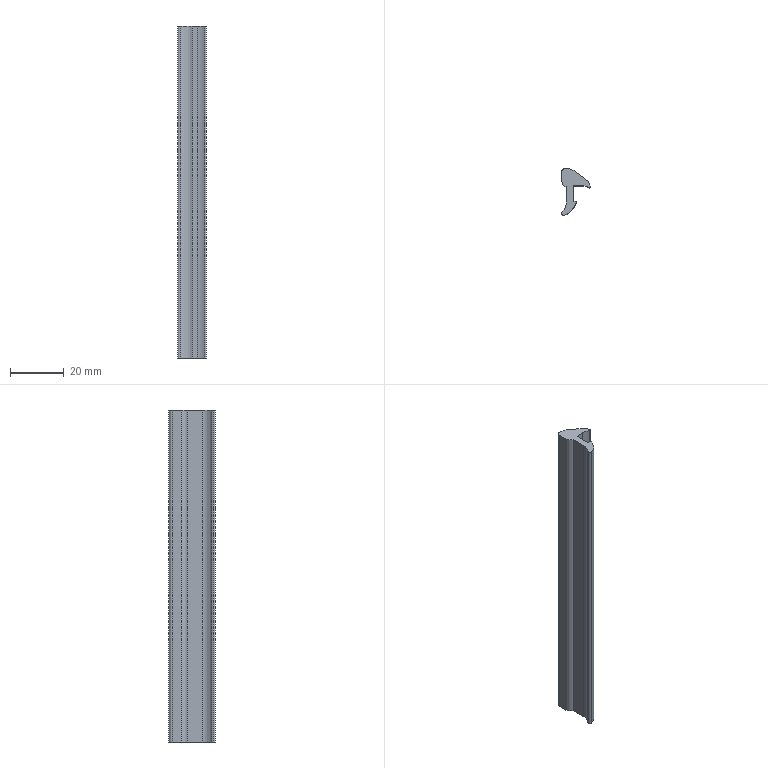Part | SolidWorks | features MoveFace 2, BaseBody 1 | 1 solid | 20 faces | box 10.8 x 17.5 x 124 mm | volume 9771 mm3 | cylinder 11 | plane 9 | commonest cylinder face diameters 1.6 x2 14 x2 0.4 x1 0.6 x1 0.8 x1 2.6 x1
STEP:
#1=CARTESIAN_POINT('',(-3.236,-11.055,-25.));
#2=VERTEX_POINT('',#1);
#3=CARTESIAN_POINT('',(-4.3,-10.3,-25.));
#4=VERTEX_POINT('',#3);
#5=CARTESIAN_POINT('',(-3.5,-10.3,-25.));
#6=DIRECTION('',(0.,0.,-1.));
#7=DIRECTION('',(1.,0.,0.));
#8=AXIS2_PLACEMENT_3D('',#5,#6,#7);
#9=CIRCLE('',#8,0.8);
#10=EDGE_CURVE('',#2,#4,#9,.T.);
#11=ORIENTED_EDGE('',*,*,#10,.T.);
#12=CARTESIAN_POINT('',(-4.3,-10.3,-149.));
#13=VERTEX_POINT('',#12);
#14=CARTESIAN_POINT('',(-4.3,-10.3,-100.));
#15=DIRECTION('',(0.,0.,-1.));
#16=VECTOR('',#15,1000.);
#17=LINE('',#14,#16);
#18=EDGE_CURVE('',#4,#13,#17,.T.);
#19=ORIENTED_EDGE('',*,*,#18,.T.);
#20=CARTESIAN_POINT('',(-3.236,-11.055,-149.));
#21=VERTEX_POINT('',#20);
#22=CARTESIAN_POINT('',(-3.5,-10.3,-149.));
#23=DIRECTION('',(0.,0.,1.));
#24=DIRECTION('',(1.,0.,0.));
#25=AXIS2_PLACEMENT_3D('',#22,#23,#24);
#26=CIRCLE('',#25,0.8);
#27=EDGE_CURVE('',#13,#21,#26,.T.);
#28=ORIENTED_EDGE('',*,*,#27,.T.);
#29=CARTESIAN_POINT('',(-3.236,-11.055,-100.));
#30=DIRECTION('',(0.,0.,-1.));
#31=VECTOR('',#30,1000.);
#32=LINE('',#29,#31);
#33=EDGE_CURVE('',#2,#21,#32,.T.);
#34=ORIENTED_EDGE('',*,*,#33,.F.);
#35=EDGE_LOOP('',(#11,#19,#28,#34));
#36=FACE_OUTER_BOUND('',#35,.T.);
#37=CARTESIAN_POINT('',(-3.5,-10.3,-100.));
#38=DIRECTION('',(0.,0.,-1.));
#39=DIRECTION('',(-1.,0.,0.));
#40=AXIS2_PLACEMENT_3D('',#37,#38,#39);
#41=CYLINDRICAL_SURFACE('',#40,0.8);
#42=ADVANCED_FACE('',(#36),#41,.T.);
#43=CARTESIAN_POINT('',(1.184,-6.397,-149.));
#44=VERTEX_POINT('',#43);
#45=CARTESIAN_POINT('',(-5.702,-4.29,-149.));
#46=DIRECTION('',(0.,0.,1.));
#47=DIRECTION('',(1.,0.,0.));
#48=AXIS2_PLACEMENT_3D('',#45,#46,#47);
#49=CIRCLE('',#48,7.201);
#50=EDGE_CURVE('',#21,#44,#49,.T.);
#51=ORIENTED_EDGE('',*,*,#50,.T.);
#52=CARTESIAN_POINT('',(1.184,-6.397,-25.));
#53=VERTEX_POINT('',#52);
#54=CARTESIAN_POINT('',(1.184,-6.397,-100.));
#55=DIRECTION('',(0.,0.,1.));
#56=VECTOR('',#55,1000.);
#57=LINE('',#54,#56);
#58=EDGE_CURVE('',#44,#53,#57,.T.);
#59=ORIENTED_EDGE('',*,*,#58,.T.);
#60=CARTESIAN_POINT('',(-5.702,-4.29,-25.));
#61=DIRECTION('',(0.,0.,-1.));
#62=DIRECTION('',(1.,0.,0.));
#63=AXIS2_PLACEMENT_3D('',#60,#61,#62);
#64=CIRCLE('',#63,7.201);
#65=EDGE_CURVE('',#53,#2,#64,.T.);
#66=ORIENTED_EDGE('',*,*,#65,.T.);
#67=ORIENTED_EDGE('',*,*,#33,.T.);
#68=EDGE_LOOP('',(#51,#59,#66,#67));
#69=FACE_OUTER_BOUND('',#68,.T.);
#70=CARTESIAN_POINT('',(-5.702,-4.29,-100.));
#71=DIRECTION('',(0.,0.,-1.));
#72=DIRECTION('',(-1.,0.,0.));
#73=AXIS2_PLACEMENT_3D('',#70,#71,#72);
#74=CYLINDRICAL_SURFACE('',#73,7.201);
#75=ADVANCED_FACE('',(#69),#74,.T.);
#76=CARTESIAN_POINT('',(0.9,-6.,-149.));
#77=VERTEX_POINT('',#76);
#78=CARTESIAN_POINT('',(0.9,-6.3,-149.));
#79=DIRECTION('',(0.,0.,1.));
#80=DIRECTION('',(1.,0.,0.));
#81=AXIS2_PLACEMENT_3D('',#78,#79,#80);
#82=CIRCLE('',#81,0.3);
#83=EDGE_CURVE('',#44,#77,#82,.T.);
#84=ORIENTED_EDGE('',*,*,#83,.T.);
#85=CARTESIAN_POINT('',(0.9,-6.,-25.));
#86=VERTEX_POINT('',#85);
#87=CARTESIAN_POINT('',(0.9,-6.,-100.));
#88=DIRECTION('',(0.,0.,1.));
#89=VECTOR('',#88,1000.);
#90=LINE('',#87,#89);
#91=EDGE_CURVE('',#77,#86,#90,.T.);
#92=ORIENTED_EDGE('',*,*,#91,.T.);
#93=CARTESIAN_POINT('',(0.9,-6.3,-25.));
#94=DIRECTION('',(0.,0.,-1.));
#95=DIRECTION('',(1.,0.,0.));
#96=AXIS2_PLACEMENT_3D('',#93,#94,#95);
#97=CIRCLE('',#96,0.3);
#98=EDGE_CURVE('',#86,#53,#97,.T.);
#99=ORIENTED_EDGE('',*,*,#98,.T.);
#100=ORIENTED_EDGE('',*,*,#58,.F.);
#101=EDGE_LOOP('',(#84,#92,#99,#100));
#102=FACE_OUTER_BOUND('',#101,.T.);
#103=CARTESIAN_POINT('',(0.9,-6.3,-100.));
#104=DIRECTION('',(0.,0.,-1.));
#105=DIRECTION('',(-1.,0.,0.));
#106=AXIS2_PLACEMENT_3D('',#103,#104,#105);
#107=CYLINDRICAL_SURFACE('',#106,0.3);
#108=ADVANCED_FACE('',(#102),#107,.T.);
#109=CARTESIAN_POINT('',(-2.5,-0.5,-149.));
#110=VERTEX_POINT('',#109);
#111=CARTESIAN_POINT('',(-2.5,-6.153,-149.));
#112=VERTEX_POINT('',#111);
#113=CARTESIAN_POINT('',(-2.5,-6.397,-149.));
#114=DIRECTION('',(0.,-1.,0.));
#115=VECTOR('',#114,1000.);
#116=LINE('',#113,#115);
#117=EDGE_CURVE('',#110,#112,#116,.T.);
#118=ORIENTED_EDGE('',*,*,#117,.F.);
#119=CARTESIAN_POINT('',(-4.2,1.695,-149.));
#120=VERTEX_POINT('',#119);
#121=CARTESIAN_POINT('',(-1.701,1.875,-149.));
#122=DIRECTION('',(0.,0.,1.));
#123=DIRECTION('',(1.,0.,0.));
#124=AXIS2_PLACEMENT_3D('',#121,#122,#123);
#125=CIRCLE('',#124,2.506);
#126=EDGE_CURVE('',#120,#110,#125,.T.);
#127=ORIENTED_EDGE('',*,*,#126,.F.);
#128=CARTESIAN_POINT('',(-4.2,5.1,-149.));
#129=VERTEX_POINT('',#128);
#130=CARTESIAN_POINT('',(-4.2,-6.397,-149.));
#131=DIRECTION('',(0.,-1.,0.));
#132=VECTOR('',#131,1000.);
#133=LINE('',#130,#132);
#134=EDGE_CURVE('',#129,#120,#133,.T.);
#135=ORIENTED_EDGE('',*,*,#134,.F.);
#136=CARTESIAN_POINT('',(-2.892,6.4,-149.));
#137=VERTEX_POINT('',#136);
#138=CARTESIAN_POINT('',(-2.9,5.1,-149.));
#139=DIRECTION('',(0.,0.,1.));
#140=DIRECTION('',(1.,0.,0.));
#141=AXIS2_PLACEMENT_3D('',#138,#139,#140);
#142=CIRCLE('',#141,1.3);
#143=EDGE_CURVE('',#137,#129,#142,.T.);
#144=ORIENTED_EDGE('',*,*,#143,.F.);
#145=CARTESIAN_POINT('',(0.5,5.5,-149.));
#146=VERTEX_POINT('',#145);
#147=CARTESIAN_POINT('',(-2.934,-0.5999,-149.));
#148=DIRECTION('',(0.,0.,1.));
#149=DIRECTION('',(1.,0.,0.));
#150=AXIS2_PLACEMENT_3D('',#147,#148,#149);
#151=CIRCLE('',#150,7.);
#152=EDGE_CURVE('',#146,#137,#151,.T.);
#153=ORIENTED_EDGE('',*,*,#152,.F.);
#154=CARTESIAN_POINT('',(5.5,1.7,-149.));
#155=VERTEX_POINT('',#154);
#156=CARTESIAN_POINT('',(1.595,4.668,-149.));
#157=DIRECTION('',(-0.7962,0.6051,0.));
#158=VECTOR('',#157,1000.);
#159=LINE('',#156,#158);
#160=EDGE_CURVE('',#155,#146,#159,.T.);
#161=ORIENTED_EDGE('',*,*,#160,.F.);
#162=CARTESIAN_POINT('',(6.458,-0.2215,-149.));
#163=VERTEX_POINT('',#162);
#164=CARTESIAN_POINT('',(6.282,0.1323,-149.));
#165=DIRECTION('',(-0.4462,0.8949,0.));
#166=VECTOR('',#165,1000.);
#167=LINE('',#164,#166);
#168=EDGE_CURVE('',#163,#155,#167,.T.);
#169=ORIENTED_EDGE('',*,*,#168,.F.);
#170=CARTESIAN_POINT('',(5.895,-0.7433,-149.));
#171=VERTEX_POINT('',#170);
#172=CARTESIAN_POINT('',(6.1,-0.4,-149.));
#173=DIRECTION('',(0.,0.,1.));
#174=DIRECTION('',(1.,0.,0.));
#175=AXIS2_PLACEMENT_3D('',#172,#173,#174);
#176=CIRCLE('',#175,0.4);
#177=EDGE_CURVE('',#171,#163,#176,.T.);
#178=ORIENTED_EDGE('',*,*,#177,.F.);
#179=CARTESIAN_POINT('',(3.,0.,-149.));
#180=VERTEX_POINT('',#179);
#181=CARTESIAN_POINT('',(2.746,-6.995,-149.));
#182=DIRECTION('',(0.,0.,-1.));
#183=DIRECTION('',(1.,0.,0.));
#184=AXIS2_PLACEMENT_3D('',#181,#182,#183);
#185=CIRCLE('',#184,7.);
#186=EDGE_CURVE('',#180,#171,#185,.T.);
#187=ORIENTED_EDGE('',*,*,#186,.F.);
#188=CARTESIAN_POINT('',(0.,0.,-149.));
#189=VERTEX_POINT('',#188);
#190=CARTESIAN_POINT('',(-6.814,0.,-149.));
#191=DIRECTION('',(1.,0.,0.));
#192=VECTOR('',#191,1000.);
#193=LINE('',#190,#192);
#194=EDGE_CURVE('',#189,#180,#193,.T.);
#195=ORIENTED_EDGE('',*,*,#194,.F.);
#196=CARTESIAN_POINT('',(0.,-5.8,-149.));
#197=VERTEX_POINT('',#196);
#198=CARTESIAN_POINT('',(0.,-6.397,-149.));
#199=DIRECTION('',(0.,1.,0.));
#200=VECTOR('',#199,1000.);
#201=LINE('',#198,#200);
#202=EDGE_CURVE('',#197,#189,#201,.T.);
#203=ORIENTED_EDGE('',*,*,#202,.F.);
#204=CARTESIAN_POINT('',(0.2,-6.,-149.));
#205=VERTEX_POINT('',#204);
#206=CARTESIAN_POINT('',(0.2,-5.8,-149.));
#207=DIRECTION('',(0.,0.,1.));
#208=DIRECTION('',(1.,0.,0.));
#209=AXIS2_PLACEMENT_3D('',#206,#207,#208);
#210=CIRCLE('',#209,0.2);
#211=EDGE_CURVE('',#197,#205,#210,.T.);
#212=ORIENTED_EDGE('',*,*,#211,.T.);
#213=CARTESIAN_POINT('',(-6.814,-6.,-149.));
#214=DIRECTION('',(-1.,0.,0.));
#215=VECTOR('',#214,1000.);
#216=LINE('',#213,#215);
#217=EDGE_CURVE('',#77,#205,#216,.T.);
#218=ORIENTED_EDGE('',*,*,#217,.F.);
#219=ORIENTED_EDGE('',*,*,#83,.F.);
#220=ORIENTED_EDGE('',*,*,#50,.F.);
#221=ORIENTED_EDGE('',*,*,#27,.F.);
#222=CARTESIAN_POINT('',(-3.998,-9.674,-149.));
#223=VERTEX_POINT('',#222);
#224=CARTESIAN_POINT('',(-3.5,-10.3,-149.));
#225=DIRECTION('',(0.,0.,1.));
#226=DIRECTION('',(1.,0.,0.));
#227=AXIS2_PLACEMENT_3D('',#224,#225,#226);
#228=CIRCLE('',#227,0.8);
#229=EDGE_CURVE('',#223,#13,#228,.T.);
#230=ORIENTED_EDGE('',*,*,#229,.F.);
#231=CARTESIAN_POINT('',(-6.814,-6.397,-149.));
#232=DIRECTION('',(0.,0.,-1.));
#233=DIRECTION('',(1.,0.,0.));
#234=AXIS2_PLACEMENT_3D('',#231,#232,#233);
#235=CIRCLE('',#234,4.321);
#236=EDGE_CURVE('',#112,#223,#235,.T.);
#237=ORIENTED_EDGE('',*,*,#236,.F.);
#238=EDGE_LOOP('',(#118,#127,#135,#144,#153,#161,#169,#178,#187,#195,#203,#212,#218,#219,#220,#221,#230,#237));
#239=FACE_OUTER_BOUND('',#238,.T.);
#240=CARTESIAN_POINT('',(-6.814,-6.397,-149.));
#241=DIRECTION('',(0.,0.,1.));
#242=DIRECTION('',(1.,0.,0.));
#243=AXIS2_PLACEMENT_3D('',#240,#241,#242);
#244=PLANE('',#243);
#245=ADVANCED_FACE('',(#239),#244,.F.);
#246=ORIENTED_EDGE('',*,*,#18,.F.);
#247=CARTESIAN_POINT('',(-3.998,-9.674,-25.));
#248=VERTEX_POINT('',#247);
#249=CARTESIAN_POINT('',(-3.5,-10.3,-25.));
#250=DIRECTION('',(0.,0.,-1.));
#251=DIRECTION('',(1.,0.,0.));
#252=AXIS2_PLACEMENT_3D('',#249,#250,#251);
#253=CIRCLE('',#252,0.8);
#254=EDGE_CURVE('',#4,#248,#253,.T.);
#255=ORIENTED_EDGE('',*,*,#254,.T.);
#256=CARTESIAN_POINT('',(-3.998,-9.674,-100.));
#257=DIRECTION('',(0.,0.,-1.));
#258=VECTOR('',#257,1000.);
#259=LINE('',#256,#258);
#260=EDGE_CURVE('',#248,#223,#259,.T.);
#261=ORIENTED_EDGE('',*,*,#260,.T.);
#262=ORIENTED_EDGE('',*,*,#229,.T.);
#263=EDGE_LOOP('',(#246,#255,#261,#262));
#264=FACE_OUTER_BOUND('',#263,.T.);
#265=CARTESIAN_POINT('',(-3.5,-10.3,-100.));
#266=DIRECTION('',(0.,0.,-1.));
#267=DIRECTION('',(-1.,0.,0.));
#268=AXIS2_PLACEMENT_3D('',#265,#266,#267);
#269=CYLINDRICAL_SURFACE('',#268,0.8);
#270=ADVANCED_FACE('',(#264),#269,.T.);
#271=CARTESIAN_POINT('',(-4.2,1.695,-25.));
#272=VERTEX_POINT('',#271);
#273=CARTESIAN_POINT('',(-2.5,-0.5,-25.));
#274=VERTEX_POINT('',#273);
#275=CARTESIAN_POINT('',(-1.701,1.875,-25.));
#276=DIRECTION('',(0.,0.,1.));
#277=DIRECTION('',(1.,0.,0.));
#278=AXIS2_PLACEMENT_3D('',#275,#276,#277);
#279=CIRCLE('',#278,2.506);
#280=EDGE_CURVE('',#272,#274,#279,.T.);
#281=ORIENTED_EDGE('',*,*,#280,.T.);
#282=CARTESIAN_POINT('',(-2.5,-6.153,-25.));
#283=VERTEX_POINT('',#282);
#284=CARTESIAN_POINT('',(-2.5,-6.397,-25.));
#285=DIRECTION('',(0.,-1.,0.));
#286=VECTOR('',#285,1000.);
#287=LINE('',#284,#286);
#288=EDGE_CURVE('',#274,#283,#287,.T.);
#289=ORIENTED_EDGE('',*,*,#288,.T.);
#290=CARTESIAN_POINT('',(-6.814,-6.397,-25.));
#291=DIRECTION('',(0.,0.,-1.));
#292=DIRECTION('',(1.,0.,0.));
#293=AXIS2_PLACEMENT_3D('',#290,#291,#292);
#294=CIRCLE('',#293,4.321);
#295=EDGE_CURVE('',#283,#248,#294,.T.);
#296=ORIENTED_EDGE('',*,*,#295,.T.);
#297=ORIENTED_EDGE('',*,*,#254,.F.);
#298=ORIENTED_EDGE('',*,*,#10,.F.);
#299=ORIENTED_EDGE('',*,*,#65,.F.);
#300=ORIENTED_EDGE('',*,*,#98,.F.);
#301=CARTESIAN_POINT('',(0.2,-6.,-25.));
#302=VERTEX_POINT('',#301);
#303=CARTESIAN_POINT('',(-6.814,-6.,-25.));
#304=DIRECTION('',(-1.,0.,0.));
#305=VECTOR('',#304,1000.);
#306=LINE('',#303,#305);
#307=EDGE_CURVE('',#86,#302,#306,.T.);
#308=ORIENTED_EDGE('',*,*,#307,.T.);
#309=CARTESIAN_POINT('',(0.,-5.8,-25.));
#310=VERTEX_POINT('',#309);
#311=CARTESIAN_POINT('',(0.2,-5.8,-25.));
#312=DIRECTION('',(0.,0.,-1.));
#313=DIRECTION('',(1.,0.,0.));
#314=AXIS2_PLACEMENT_3D('',#311,#312,#313);
#315=CIRCLE('',#314,0.2);
#316=EDGE_CURVE('',#302,#310,#315,.T.);
#317=ORIENTED_EDGE('',*,*,#316,.T.);
#318=CARTESIAN_POINT('',(0.,0.,-25.));
#319=VERTEX_POINT('',#318);
#320=CARTESIAN_POINT('',(0.,-6.397,-25.));
#321=DIRECTION('',(0.,1.,0.));
#322=VECTOR('',#321,1000.);
#323=LINE('',#320,#322);
#324=EDGE_CURVE('',#310,#319,#323,.T.);
#325=ORIENTED_EDGE('',*,*,#324,.T.);
#326=CARTESIAN_POINT('',(3.,0.,-25.));
#327=VERTEX_POINT('',#326);
#328=CARTESIAN_POINT('',(-6.814,0.,-25.));
#329=DIRECTION('',(1.,0.,0.));
#330=VECTOR('',#329,1000.);
#331=LINE('',#328,#330);
#332=EDGE_CURVE('',#319,#327,#331,.T.);
#333=ORIENTED_EDGE('',*,*,#332,.T.);
#334=CARTESIAN_POINT('',(5.895,-0.7433,-25.));
#335=VERTEX_POINT('',#334);
#336=CARTESIAN_POINT('',(2.746,-6.995,-25.));
#337=DIRECTION('',(0.,0.,-1.));
#338=DIRECTION('',(1.,0.,0.));
#339=AXIS2_PLACEMENT_3D('',#336,#337,#338);
#340=CIRCLE('',#339,7.);
#341=EDGE_CURVE('',#327,#335,#340,.T.);
#342=ORIENTED_EDGE('',*,*,#341,.T.);
#343=CARTESIAN_POINT('',(6.458,-0.2215,-25.));
#344=VERTEX_POINT('',#343);
#345=CARTESIAN_POINT('',(6.1,-0.4,-25.));
#346=DIRECTION('',(0.,0.,-1.));
#347=DIRECTION('',(1.,0.,0.));
#348=AXIS2_PLACEMENT_3D('',#345,#346,#347);
#349=CIRCLE('',#348,0.4);
#350=EDGE_CURVE('',#344,#335,#349,.T.);
#351=ORIENTED_EDGE('',*,*,#350,.F.);
#352=CARTESIAN_POINT('',(5.5,1.7,-25.));
#353=VERTEX_POINT('',#352);
#354=CARTESIAN_POINT('',(6.282,0.1323,-25.));
#355=DIRECTION('',(-0.4462,0.8949,0.));
#356=VECTOR('',#355,1000.);
#357=LINE('',#354,#356);
#358=EDGE_CURVE('',#344,#353,#357,.T.);
#359=ORIENTED_EDGE('',*,*,#358,.T.);
#360=CARTESIAN_POINT('',(0.5,5.5,-25.));
#361=VERTEX_POINT('',#360);
#362=CARTESIAN_POINT('',(1.595,4.668,-25.));
#363=DIRECTION('',(-0.7962,0.6051,0.));
#364=VECTOR('',#363,1000.);
#365=LINE('',#362,#364);
#366=EDGE_CURVE('',#353,#361,#365,.T.);
#367=ORIENTED_EDGE('',*,*,#366,.T.);
#368=CARTESIAN_POINT('',(-2.892,6.4,-25.));
#369=VERTEX_POINT('',#368);
#370=CARTESIAN_POINT('',(-2.934,-0.5999,-25.));
#371=DIRECTION('',(0.,0.,1.));
#372=DIRECTION('',(1.,0.,0.));
#373=AXIS2_PLACEMENT_3D('',#370,#371,#372);
#374=CIRCLE('',#373,7.);
#375=EDGE_CURVE('',#361,#369,#374,.T.);
#376=ORIENTED_EDGE('',*,*,#375,.T.);
#377=CARTESIAN_POINT('',(-4.2,5.1,-25.));
#378=VERTEX_POINT('',#377);
#379=CARTESIAN_POINT('',(-2.9,5.1,-25.));
#380=DIRECTION('',(0.,0.,1.));
#381=DIRECTION('',(1.,0.,0.));
#382=AXIS2_PLACEMENT_3D('',#379,#380,#381);
#383=CIRCLE('',#382,1.3);
#384=EDGE_CURVE('',#369,#378,#383,.T.);
#385=ORIENTED_EDGE('',*,*,#384,.T.);
#386=CARTESIAN_POINT('',(-4.2,-6.397,-25.));
#387=DIRECTION('',(0.,-1.,0.));
#388=VECTOR('',#387,1000.);
#389=LINE('',#386,#388);
#390=EDGE_CURVE('',#378,#272,#389,.T.);
#391=ORIENTED_EDGE('',*,*,#390,.T.);
#392=EDGE_LOOP('',(#281,#289,#296,#297,#298,#299,#300,#308,#317,#325,#333,#342,#351,#359,#367,#376,#385,#391));
#393=FACE_OUTER_BOUND('',#392,.T.);
#394=CARTESIAN_POINT('',(-6.814,-6.397,-25.));
#395=DIRECTION('',(0.,0.,1.));
#396=DIRECTION('',(1.,0.,0.));
#397=AXIS2_PLACEMENT_3D('',#394,#395,#396);
#398=PLANE('',#397);
#399=ADVANCED_FACE('',(#393),#398,.T.);
#400=ORIENTED_EDGE('',*,*,#217,.T.);
#401=CARTESIAN_POINT('',(0.2,-6.,-100.));
#402=DIRECTION('',(0.,0.,1.));
#403=VECTOR('',#402,1000.);
#404=LINE('',#401,#403);
#405=EDGE_CURVE('',#205,#302,#404,.T.);
#406=ORIENTED_EDGE('',*,*,#405,.T.);
#407=ORIENTED_EDGE('',*,*,#307,.F.);
#408=ORIENTED_EDGE('',*,*,#91,.F.);
#409=EDGE_LOOP('',(#400,#406,#407,#408));
#410=FACE_OUTER_BOUND('',#409,.T.);
#411=CARTESIAN_POINT('',(0.9,-6.,-100.));
#412=DIRECTION('',(0.,1.,0.));
#413=DIRECTION('',(0.,0.,1.));
#414=AXIS2_PLACEMENT_3D('',#411,#412,#413);
#415=PLANE('',#414);
#416=ADVANCED_FACE('',(#410),#415,.T.);
#417=CARTESIAN_POINT('',(-2.5,-6.153,-100.));
#418=DIRECTION('',(0.,0.,1.));
#419=VECTOR('',#418,1000.);
#420=LINE('',#417,#419);
#421=EDGE_CURVE('',#112,#283,#420,.T.);
#422=ORIENTED_EDGE('',*,*,#421,.F.);
#423=ORIENTED_EDGE('',*,*,#236,.T.);
#424=ORIENTED_EDGE('',*,*,#260,.F.);
#425=ORIENTED_EDGE('',*,*,#295,.F.);
#426=EDGE_LOOP('',(#422,#423,#424,#425));
#427=FACE_OUTER_BOUND('',#426,.T.);
#428=CARTESIAN_POINT('',(-6.814,-6.397,-100.));
#429=DIRECTION('',(0.,0.,-1.));
#430=DIRECTION('',(-1.,0.,0.));
#431=AXIS2_PLACEMENT_3D('',#428,#429,#430);
#432=CYLINDRICAL_SURFACE('',#431,4.321);
#433=ADVANCED_FACE('',(#427),#432,.F.);
#434=ORIENTED_EDGE('',*,*,#117,.T.);
#435=ORIENTED_EDGE('',*,*,#421,.T.);
#436=ORIENTED_EDGE('',*,*,#288,.F.);
#437=CARTESIAN_POINT('',(-2.5,-0.5,-100.));
#438=DIRECTION('',(0.,0.,-1.));
#439=VECTOR('',#438,1000.);
#440=LINE('',#437,#439);
#441=EDGE_CURVE('',#274,#110,#440,.T.);
#442=ORIENTED_EDGE('',*,*,#441,.T.);
#443=EDGE_LOOP('',(#434,#435,#436,#442));
#444=FACE_OUTER_BOUND('',#443,.T.);
#445=CARTESIAN_POINT('',(-2.5,-0.5,-100.));
#446=DIRECTION('',(-1.,0.,0.));
#447=DIRECTION('',(0.,0.,1.));
#448=AXIS2_PLACEMENT_3D('',#445,#446,#447);
#449=PLANE('',#448);
#450=ADVANCED_FACE('',(#444),#449,.T.);
#451=ORIENTED_EDGE('',*,*,#126,.T.);
#452=ORIENTED_EDGE('',*,*,#441,.F.);
#453=ORIENTED_EDGE('',*,*,#280,.F.);
#454=CARTESIAN_POINT('',(-4.2,1.695,-100.));
#455=DIRECTION('',(0.,0.,-1.));
#456=VECTOR('',#455,1000.);
#457=LINE('',#454,#456);
#458=EDGE_CURVE('',#272,#120,#457,.T.);
#459=ORIENTED_EDGE('',*,*,#458,.T.);
#460=EDGE_LOOP('',(#451,#452,#453,#459));
#461=FACE_OUTER_BOUND('',#460,.T.);
#462=CARTESIAN_POINT('',(-1.701,1.875,-100.));
#463=DIRECTION('',(0.,0.,-1.));
#464=DIRECTION('',(-1.,0.,0.));
#465=AXIS2_PLACEMENT_3D('',#462,#463,#464);
#466=CYLINDRICAL_SURFACE('',#465,2.506);
#467=ADVANCED_FACE('',(#461),#466,.T.);
#468=ORIENTED_EDGE('',*,*,#134,.T.);
#469=ORIENTED_EDGE('',*,*,#458,.F.);
#470=ORIENTED_EDGE('',*,*,#390,.F.);
#471=CARTESIAN_POINT('',(-4.2,5.1,-100.));
#472=DIRECTION('',(0.,0.,-1.));
#473=VECTOR('',#472,1000.);
#474=LINE('',#471,#473);
#475=EDGE_CURVE('',#378,#129,#474,.T.);
#476=ORIENTED_EDGE('',*,*,#475,.T.);
#477=EDGE_LOOP('',(#468,#469,#470,#476));
#478=FACE_OUTER_BOUND('',#477,.T.);
#479=CARTESIAN_POINT('',(-4.2,5.1,-100.));
#480=DIRECTION('',(-1.,0.,0.));
#481=DIRECTION('',(0.,0.,1.));
#482=AXIS2_PLACEMENT_3D('',#479,#480,#481);
#483=PLANE('',#482);
#484=ADVANCED_FACE('',(#478),#483,.T.);
#485=ORIENTED_EDGE('',*,*,#143,.T.);
#486=ORIENTED_EDGE('',*,*,#475,.F.);
#487=ORIENTED_EDGE('',*,*,#384,.F.);
#488=CARTESIAN_POINT('',(-2.892,6.4,-100.));
#489=DIRECTION('',(0.,0.,-1.));
#490=VECTOR('',#489,1000.);
#491=LINE('',#488,#490);
#492=EDGE_CURVE('',#369,#137,#491,.T.);
#493=ORIENTED_EDGE('',*,*,#492,.T.);
#494=EDGE_LOOP('',(#485,#486,#487,#493));
#495=FACE_OUTER_BOUND('',#494,.T.);
#496=CARTESIAN_POINT('',(-2.9,5.1,-100.));
#497=DIRECTION('',(0.,0.,-1.));
#498=DIRECTION('',(-1.,0.,0.));
#499=AXIS2_PLACEMENT_3D('',#496,#497,#498);
#500=CYLINDRICAL_SURFACE('',#499,1.3);
#501=ADVANCED_FACE('',(#495),#500,.T.);
#502=ORIENTED_EDGE('',*,*,#152,.T.);
#503=ORIENTED_EDGE('',*,*,#492,.F.);
#504=ORIENTED_EDGE('',*,*,#375,.F.);
#505=CARTESIAN_POINT('',(0.5,5.5,-100.));
#506=DIRECTION('',(0.,0.,-1.));
#507=VECTOR('',#506,1000.);
#508=LINE('',#505,#507);
#509=EDGE_CURVE('',#361,#146,#508,.T.);
#510=ORIENTED_EDGE('',*,*,#509,.T.);
#511=EDGE_LOOP('',(#502,#503,#504,#510));
#512=FACE_OUTER_BOUND('',#511,.T.);
#513=CARTESIAN_POINT('',(-2.934,-0.5999,-100.));
#514=DIRECTION('',(0.,0.,-1.));
#515=DIRECTION('',(-1.,0.,0.));
#516=AXIS2_PLACEMENT_3D('',#513,#514,#515);
#517=CYLINDRICAL_SURFACE('',#516,7.);
#518=ADVANCED_FACE('',(#512),#517,.T.);
#519=ORIENTED_EDGE('',*,*,#160,.T.);
#520=ORIENTED_EDGE('',*,*,#509,.F.);
#521=ORIENTED_EDGE('',*,*,#366,.F.);
#522=CARTESIAN_POINT('',(5.5,1.7,-100.));
#523=DIRECTION('',(0.,0.,-1.));
#524=VECTOR('',#523,1000.);
#525=LINE('',#522,#524);
#526=EDGE_CURVE('',#353,#155,#525,.T.);
#527=ORIENTED_EDGE('',*,*,#526,.T.);
#528=EDGE_LOOP('',(#519,#520,#521,#527));
#529=FACE_OUTER_BOUND('',#528,.T.);
#530=CARTESIAN_POINT('',(5.5,1.7,-100.));
#531=DIRECTION('',(0.6051,0.7962,0.));
#532=DIRECTION('',(-0.7962,0.6051,0.));
#533=AXIS2_PLACEMENT_3D('',#530,#531,#532);
#534=PLANE('',#533);
#535=ADVANCED_FACE('',(#529),#534,.T.);
#536=ORIENTED_EDGE('',*,*,#168,.T.);
#537=ORIENTED_EDGE('',*,*,#526,.F.);
#538=ORIENTED_EDGE('',*,*,#358,.F.);
#539=CARTESIAN_POINT('',(6.458,-0.2215,-100.));
#540=DIRECTION('',(0.,0.,-1.));
#541=VECTOR('',#540,1000.);
#542=LINE('',#539,#541);
#543=EDGE_CURVE('',#344,#163,#542,.T.);
#544=ORIENTED_EDGE('',*,*,#543,.T.);
#545=EDGE_LOOP('',(#536,#537,#538,#544));
#546=FACE_OUTER_BOUND('',#545,.T.);
#547=CARTESIAN_POINT('',(6.458,-0.2215,-100.));
#548=DIRECTION('',(0.8949,0.4462,0.));
#549=DIRECTION('',(-0.4462,0.8949,0.));
#550=AXIS2_PLACEMENT_3D('',#547,#548,#549);
#551=PLANE('',#550);
#552=ADVANCED_FACE('',(#546),#551,.T.);
#553=CARTESIAN_POINT('',(3.,0.,-100.));
#554=DIRECTION('',(0.,0.,1.));
#555=VECTOR('',#554,1000.);
#556=LINE('',#553,#555);
#557=EDGE_CURVE('',#180,#327,#556,.T.);
#558=ORIENTED_EDGE('',*,*,#557,.F.);
#559=ORIENTED_EDGE('',*,*,#186,.T.);
#560=CARTESIAN_POINT('',(5.895,-0.7433,-100.));
#561=DIRECTION('',(0.,0.,-1.));
#562=VECTOR('',#561,1000.);
#563=LINE('',#560,#562);
#564=EDGE_CURVE('',#335,#171,#563,.T.);
#565=ORIENTED_EDGE('',*,*,#564,.F.);
#566=ORIENTED_EDGE('',*,*,#341,.F.);
#567=EDGE_LOOP('',(#558,#559,#565,#566));
#568=FACE_OUTER_BOUND('',#567,.T.);
#569=CARTESIAN_POINT('',(2.746,-6.995,-100.));
#570=DIRECTION('',(0.,0.,-1.));
#571=DIRECTION('',(-1.,0.,0.));
#572=AXIS2_PLACEMENT_3D('',#569,#570,#571);
#573=CYLINDRICAL_SURFACE('',#572,7.);
#574=ADVANCED_FACE('',(#568),#573,.F.);
#575=ORIENTED_EDGE('',*,*,#194,.T.);
#576=ORIENTED_EDGE('',*,*,#557,.T.);
#577=ORIENTED_EDGE('',*,*,#332,.F.);
#578=CARTESIAN_POINT('',(0.,0.,-100.));
#579=DIRECTION('',(0.,0.,-1.));
#580=VECTOR('',#579,1000.);
#581=LINE('',#578,#580);
#582=EDGE_CURVE('',#319,#189,#581,.T.);
#583=ORIENTED_EDGE('',*,*,#582,.T.);
#584=EDGE_LOOP('',(#575,#576,#577,#583));
#585=FACE_OUTER_BOUND('',#584,.T.);
#586=CARTESIAN_POINT('',(0.,0.,-100.));
#587=DIRECTION('',(0.,-1.,0.));
#588=DIRECTION('',(0.,0.,-1.));
#589=AXIS2_PLACEMENT_3D('',#586,#587,#588);
#590=PLANE('',#589);
#591=ADVANCED_FACE('',(#585),#590,.T.);
#592=ORIENTED_EDGE('',*,*,#202,.T.);
#593=ORIENTED_EDGE('',*,*,#582,.F.);
#594=ORIENTED_EDGE('',*,*,#324,.F.);
#595=CARTESIAN_POINT('',(0.,-5.8,-100.));
#596=DIRECTION('',(0.,0.,-1.));
#597=VECTOR('',#596,1000.);
#598=LINE('',#595,#597);
#599=EDGE_CURVE('',#310,#197,#598,.T.);
#600=ORIENTED_EDGE('',*,*,#599,.T.);
#601=EDGE_LOOP('',(#592,#593,#594,#600));
#602=FACE_OUTER_BOUND('',#601,.T.);
#603=CARTESIAN_POINT('',(0.,-5.8,-100.));
#604=DIRECTION('',(1.,0.,0.));
#605=DIRECTION('',(0.,0.,-1.));
#606=AXIS2_PLACEMENT_3D('',#603,#604,#605);
#607=PLANE('',#606);
#608=ADVANCED_FACE('',(#602),#607,.T.);
#609=ORIENTED_EDGE('',*,*,#405,.F.);
#610=ORIENTED_EDGE('',*,*,#211,.F.);
#611=ORIENTED_EDGE('',*,*,#599,.F.);
#612=ORIENTED_EDGE('',*,*,#316,.F.);
#613=EDGE_LOOP('',(#609,#610,#611,#612));
#614=FACE_OUTER_BOUND('',#613,.T.);
#615=CARTESIAN_POINT('',(0.2,-5.8,-100.));
#616=DIRECTION('',(0.,0.,-1.));
#617=DIRECTION('',(-1.,0.,0.));
#618=AXIS2_PLACEMENT_3D('',#615,#616,#617);
#619=CYLINDRICAL_SURFACE('',#618,0.2);
#620=ADVANCED_FACE('',(#614),#619,.F.);
#621=ORIENTED_EDGE('',*,*,#177,.T.);
#622=ORIENTED_EDGE('',*,*,#543,.F.);
#623=ORIENTED_EDGE('',*,*,#350,.T.);
#624=ORIENTED_EDGE('',*,*,#564,.T.);
#625=EDGE_LOOP('',(#621,#622,#623,#624));
#626=FACE_OUTER_BOUND('',#625,.T.);
#627=CARTESIAN_POINT('',(6.1,-0.4,-100.));
#628=DIRECTION('',(0.,0.,-1.));
#629=DIRECTION('',(-1.,0.,0.));
#630=AXIS2_PLACEMENT_3D('',#627,#628,#629);
#631=CYLINDRICAL_SURFACE('',#630,0.4);
#632=ADVANCED_FACE('',(#626),#631,.T.);
#633=CLOSED_SHELL('',(#42,#75,#108,#245,#270,#399,#416,#433,#450,#467,#484,#501,#518,#535,#552,#574,#591,#608,#620,#632));
#634=MANIFOLD_SOLID_BREP('',#633);
#635=CARTESIAN_POINT('',(0.,0.,0.));
#636=DIRECTION('',(0.,0.,1.));
#637=DIRECTION('',(1.,0.,0.));
#638=AXIS2_PLACEMENT_3D('',#635,#636,#637);
#639=(LENGTH_UNIT()NAMED_UNIT(*)SI_UNIT(.MILLI.,.METRE.));
#640=UNCERTAINTY_MEASURE_WITH_UNIT(LENGTH_MEASURE(0.00001),#639,'','');
#641=(NAMED_UNIT(*)PLANE_ANGLE_UNIT()SI_UNIT($,.RADIAN.));
#642=(NAMED_UNIT(*)SI_UNIT($,.STERADIAN.)SOLID_ANGLE_UNIT());
#643=(GEOMETRIC_REPRESENTATION_CONTEXT(3)GLOBAL_UNCERTAINTY_ASSIGNED_CONTEXT((#640))GLOBAL_UNIT_ASSIGNED_CONTEXT((#639,#641,#642))REPRESENTATION_CONTEXT('',''));
#644=ADVANCED_BREP_SHAPE_REPRESENTATION('',(#634,#638),#643);